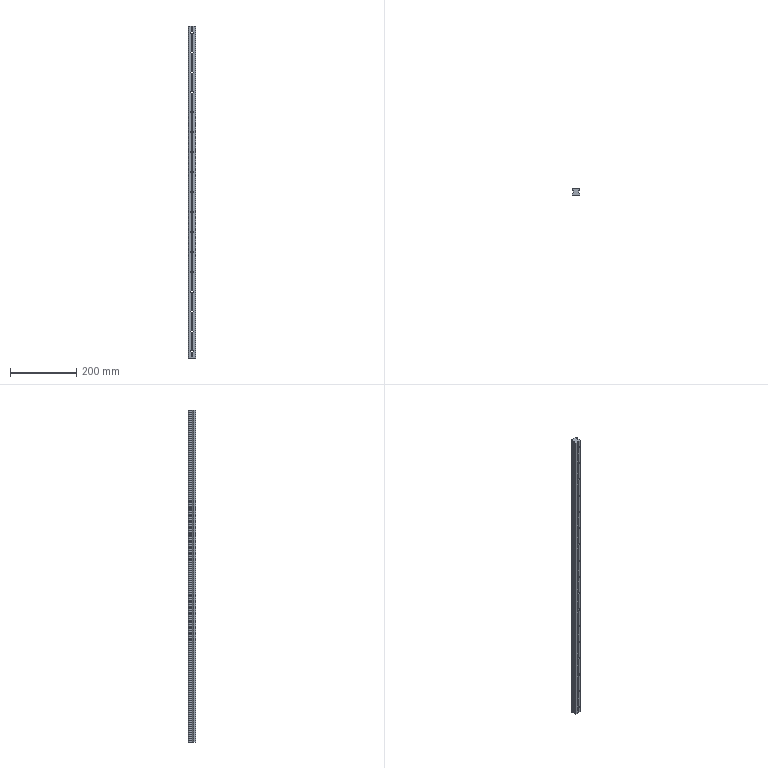Part | SolidWorks | features BaseBody 1 | 1 solid | 166 faces | box 23 x 22 x 1000 mm | volume 413117 mm3 | plane 94 | cylinder 72 | commonest cylinder face diameters 7 x34 11 x34 4.96 x4